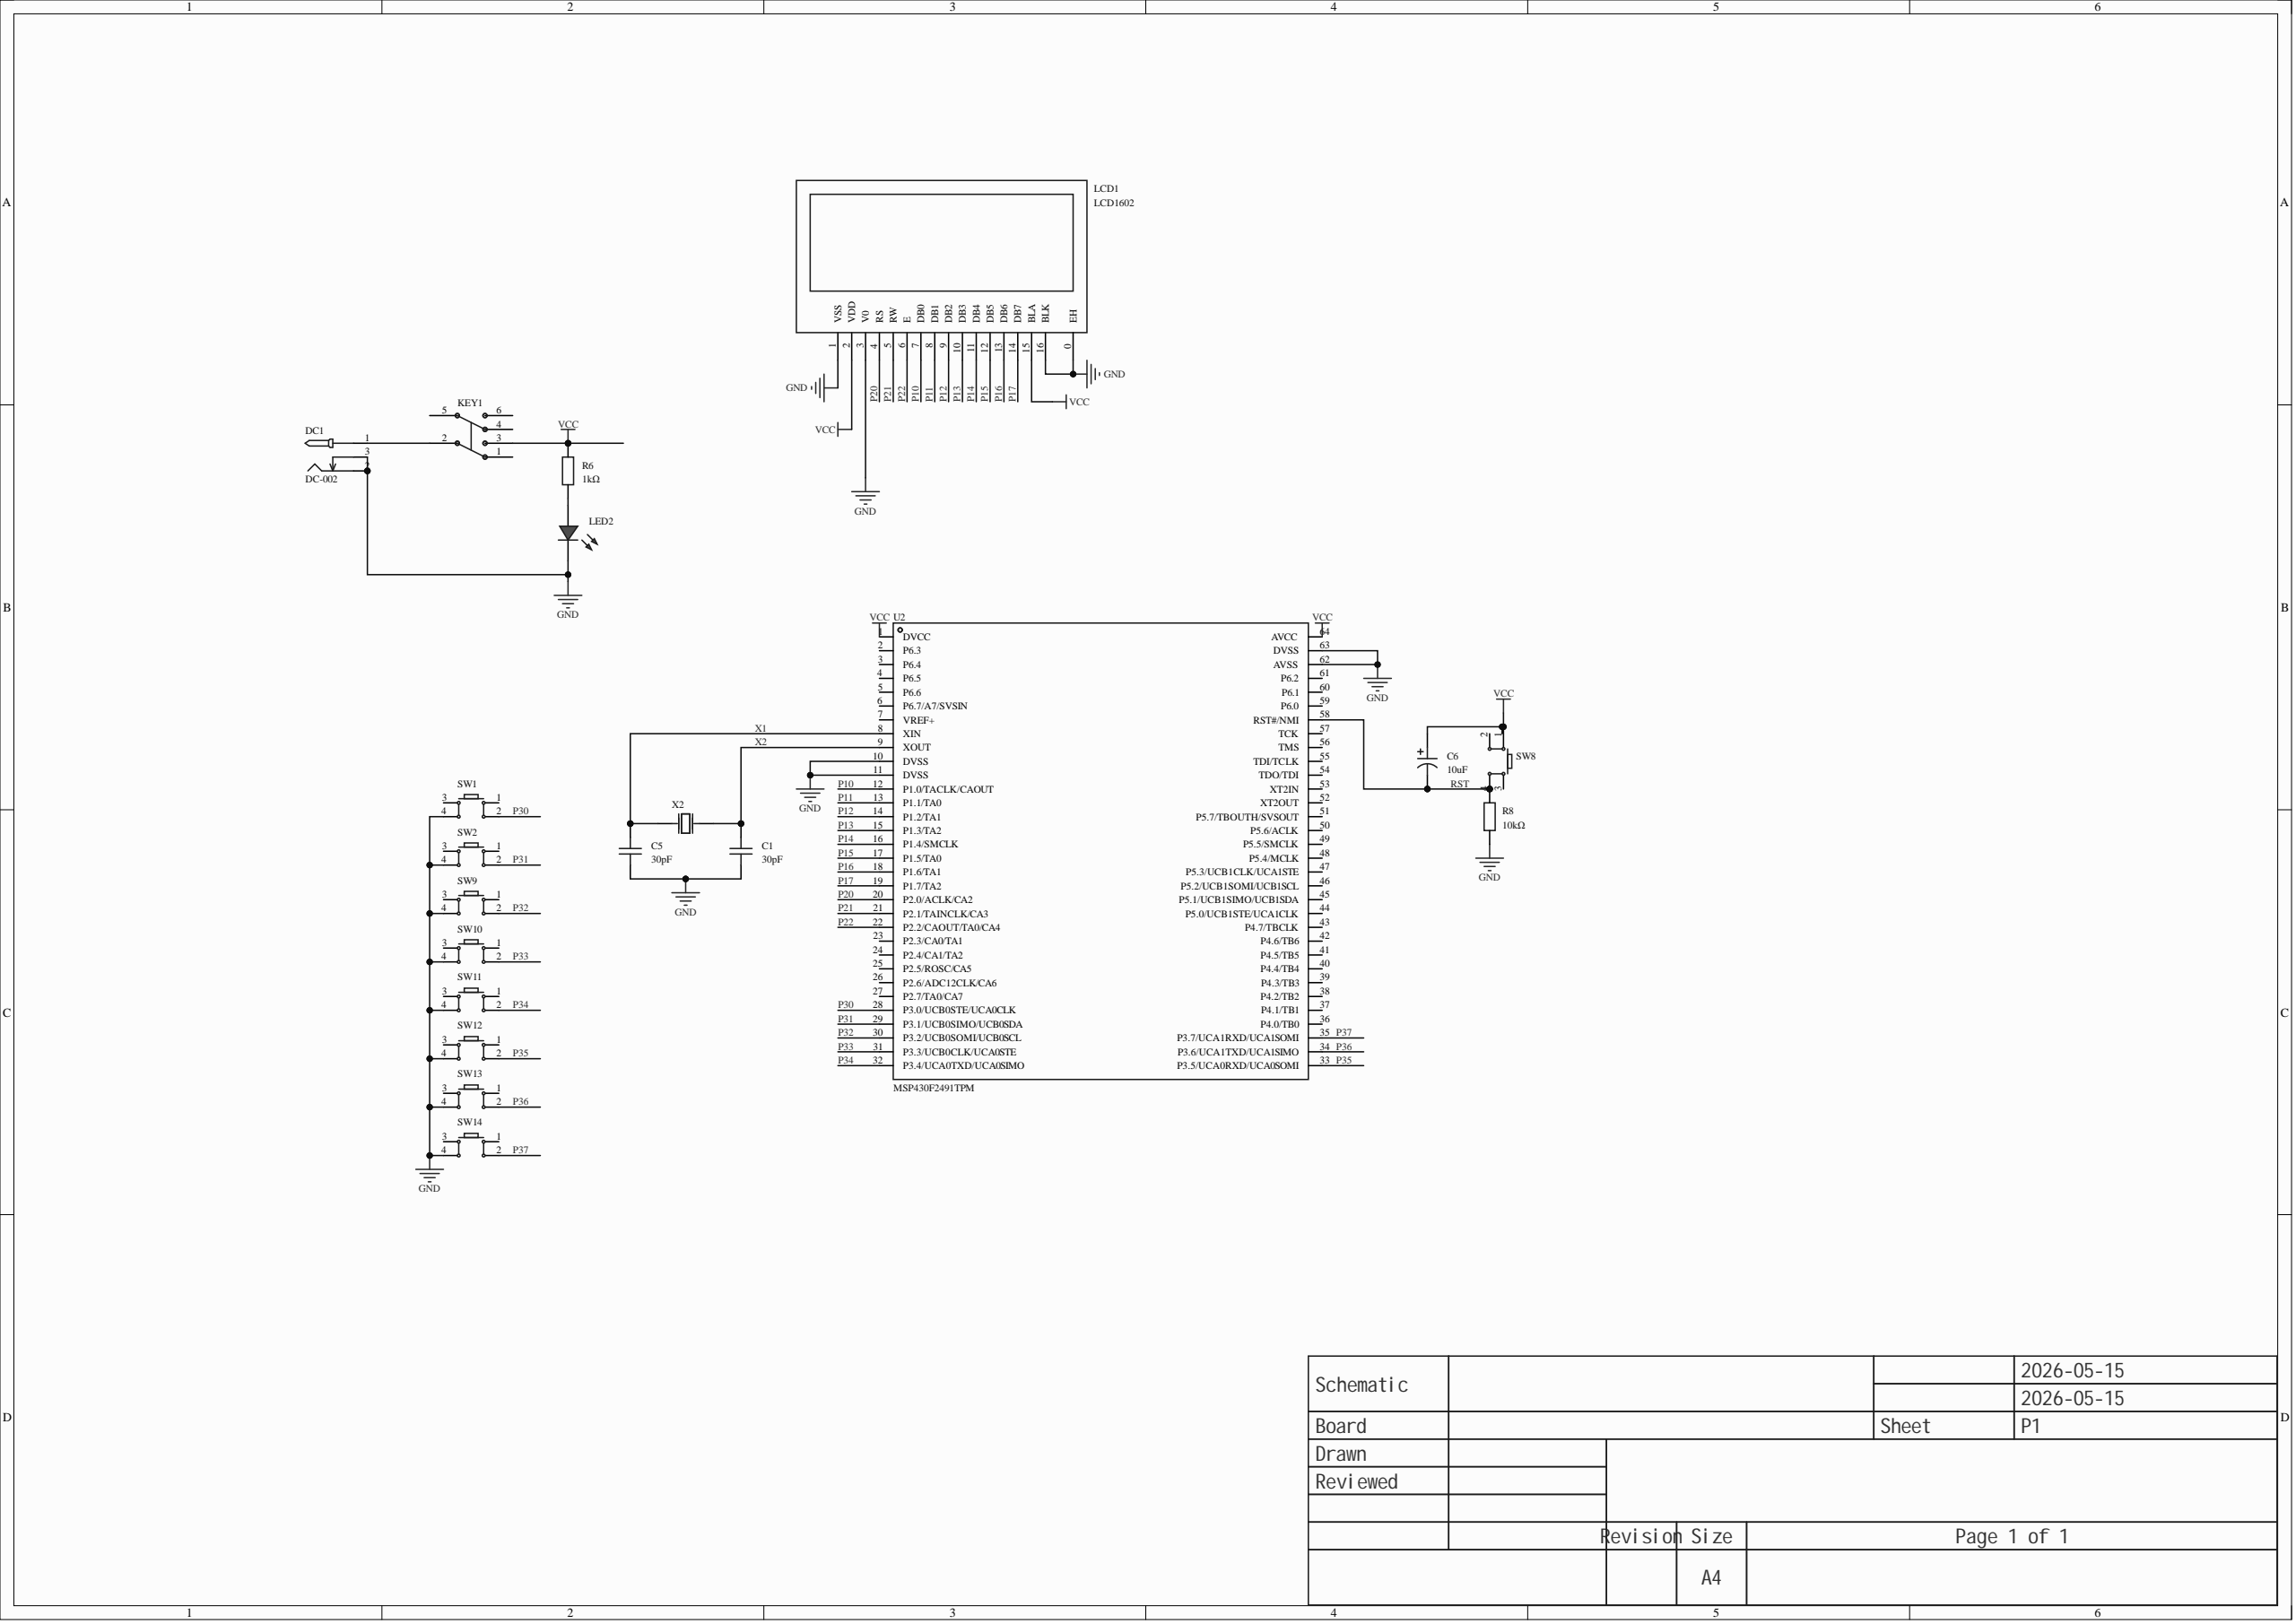Circuit board | Altium Designer | 20 parts | 26 nets
Bill of materials:
Comment,Description,Designator,Footprint,LibRef,Quantity
"30pF","Capacitance:30pF;Tolerance:±10%;Rated voltage:25V;Temperature coefficient:C0G;","C1, C5","CAP-TH_L3.8-W2.5-P2.54-D0.50","C315C300K3G5TA7301","2"
"10uF","Capacitance:10uF;Tolerance:±20%;Rated voltage:50V;Ripple current:120mA@100KHz;Equivalent series resistance (ESR):1.6Ω;","C6","CAP-TH_BD5.0-P2.00-D0.8-FD-10UF50VC110GL","10UF50VC110GL","1"
"DC-002","","DC1","DC-IN-TH_DC-3510","DC-002","1"
"Non-latching switch 8.5×8.5 silent","6 pins, 8.5×8.5","KEY1","SW-TH_6P-L8.5-W8.5-P2.54","无自锁开关 8.5×8.5 无声","1"
"LCD1602","Controller:SPLC780;Size(inch):2;","LCD1","LCD1602","HS1602A","1"
"","","LED2","LED_TH-3mm","LED_TH-R_3mm","1"
"1kΩ","","R6","Res_1/8W","Res_AXIAL-1/8W","1"
"10kΩ","","R8","Res_1/8W","Res_AXIAL-1/8W","1"
"","","SW1, SW2, SW8, SW9, SW10, SW11, SW12, SW13, SW14","SW-TH_4P-L6.0-W6.0-P4.50-LS6.5","Key_TH_6x6x6","9"
"MSP430F2491TPM","CPU core:MSP430;Program memory:60KB;Total RAM:2KB;GPIO ports:48;Operating voltage:1.8V~3.6V;CPU max frequency:16MHz;Program memory type:-;","U2","LQFP-64_L10.0-W10.0-P0.50-LS12.0-TL","MSP430F2491TPM","1"
"11.059MHz","Crystal type:Through-hole crystal;Frequency:11.059MHz;Frequency tolerance (room temp):±20ppm;Load capacitance:30pF;","X2","OSC-TH_L11.1-W4.7-P4.88","9AC11059302060C3","1"
Netlist (Protel format):
[
C1
CAP-TH_L3.8-W2.5-P2.54-D0.50
30pF



]
[
C5
CAP-TH_L3.8-W2.5-P2.54-D0.50
30pF



]
[
C6
CAP-TH_BD5.0-P2.00-D0.8-FD-10UF50VC110GL
10uF



]
[
DC1
DC-IN-TH_DC-3510
DC-002



]
[
KEY1
SW-TH_6P-L8.5-W8.5-P2.54
Non-latching switch 8.5×8.5 silent



]
[
LCD1
LCD1602
LCD1602



]
[
LED2
LED_TH-3mm




]
[
R6
Res_1/8W
1kΩ



]
[
R8
Res_1/8W
10kΩ



]
[
SW1
SW-TH_4P-L6.0-W6.0-P4.50-LS6.5




]
[
SW2
SW-TH_4P-L6.0-W6.0-P4.50-LS6.5




]
[
SW8
SW-TH_4P-L6.0-W6.0-P4.50-LS6.5




]
[
SW9
SW-TH_4P-L6.0-W6.0-P4.50-LS6.5




]
[
SW10
SW-TH_4P-L6.0-W6.0-P4.50-LS6.5




]
[
SW11
SW-TH_4P-L6.0-W6.0-P4.50-LS6.5




]
[
SW12
SW-TH_4P-L6.0-W6.0-P4.50-LS6.5




]
[
SW13
SW-TH_4P-L6.0-W6.0-P4.50-LS6.5




]
[
SW14
SW-TH_4P-L6.0-W6.0-P4.50-LS6.5




]
[
U2
LQFP-64_L10.0-W10.0-P0.50-LS12.0-TL
MSP430F2491TPM



]
[
X2
OSC-TH_L11.1-W4.7-P4.88
11.0592MHz



]
(
X2
C1-2
U2-9
X2-2
)
(
X1
C5-2
U2-8
X2-1
)
(
VCC
C6-1
KEY1-3
LCD1-2
LCD1-15
R6-2
SW8-1
U2-1
U2-64
)
(
RST
C6-2
R8-2
SW8-4
U2-58
)
(
P37
SW14-2
U2-35
)
(
P36
SW13-2
U2-34
)
(
P35
SW12-2
U2-33
)
(
P34
SW11-2
U2-32
)
(
P33
SW10-2
U2-31
)
(
P32
SW9-2
U2-30
)
(
P31
SW2-2
U2-29
)
(
P30
SW1-2
U2-28
)
(
P22
LCD1-6
U2-22
)
(
P21
LCD1-5
U2-21
)
(
P20
LCD1-4
U2-20
)
(
P17
LCD1-14
U2-19
)
(
P16
LCD1-13
U2-18
)
(
P15
LCD1-12
U2-17
)
(
P14
LCD1-11
U2-16
)
(
P13
LCD1-10
U2-15
)
(
P12
LCD1-9
U2-14
)
(
P11
LCD1-8
U2-13
)
(
P10
LCD1-7
U2-12
)
(
NetLED2_1
LED2-1
R6-1
)
(
NetDC1_1
DC1-1
KEY1-2
)
(
GND
C1-1
C5-1
DC1-2
DC1-3
LCD1-0
LCD1-1
LCD1-3
LCD1-16
LED2-2
R8-1
SW1-4
SW2-4
SW9-4
SW10-4
SW11-4
SW12-4
SW13-4
SW14-4
U2-10
U2-11
U2-62
U2-63
)